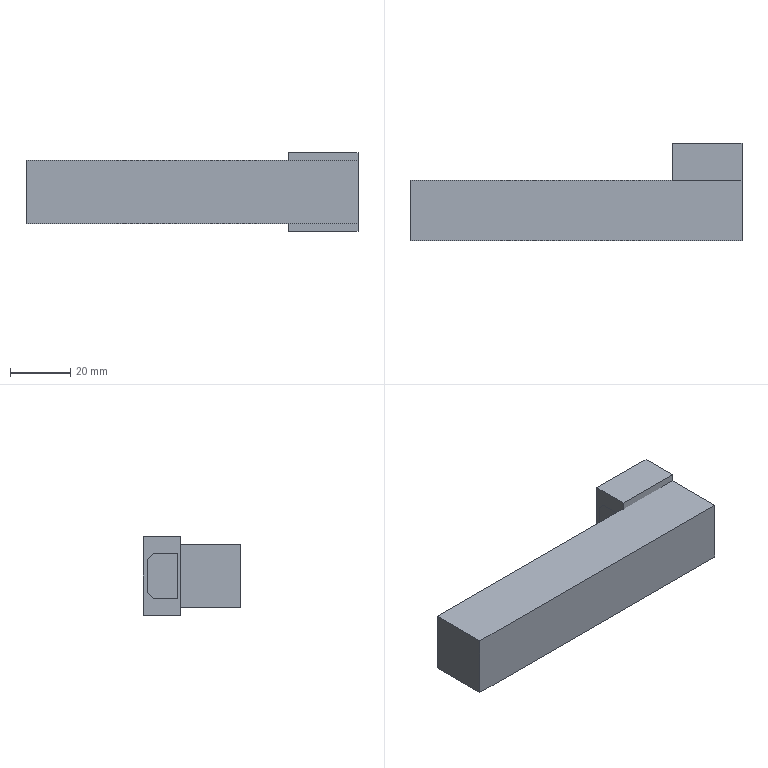NC program | NX | posted with a generic post | part box 110 x 32.2 x 26 mm
Lines 4082 to 5595 of 5595, first 1420 of 1508 lines:
(PLANAR_MILL_10 , TOOL : D4C)
N8030 T03 M6
N8032 G54
N8034 G17 G0 G90 X8.566 Y-0.32 S3000 M3
N8036 G43 Z20. H3
N8038 Z-1.8
N8040 G94 G1 X8.819 Y-0.529 Z-1.806 F1000.
N8042 X9.181 Z-1.812
N8044 X9.484 Y-0.279 Z-1.819
N8046 X9.548 Y0.108 Z-1.826
N8048 X9.367 Y0.421 Z-1.832
N8050 X9.181 Y0.529 Z-1.836
N8052 X8.819 Z-1.842
N8054 X8.633 Y0.421 Z-1.846
N8056 X8.452 Y0.108 Z-1.852
N8058 X8.516 Y-0.279 Z-1.859
N8060 X8.819 Y-0.529 Z-1.866
N8062 X9.181 Z-1.872
N8064 X9.484 Y-0.279 Z-1.879
N8066 X9.548 Y0.108 Z-1.886
N8068 X9.367 Y0.421 Z-1.892
N8070 X9.181 Y0.529 Z-1.896
N8072 X8.819 Z-1.902
N8074 X8.633 Y0.421 Z-1.906
N8076 X8.452 Y0.108 Z-1.912
N8078 X8.516 Y-0.279 Z-1.919
N8080 X8.819 Y-0.529 Z-1.926
N8082 X9.181 Z-1.932
N8084 X9.484 Y-0.279 Z-1.939
N8086 X9.548 Y0.108 Z-1.946
N8088 X9.367 Y0.421 Z-1.952
N8090 X9.181 Y0.529 Z-1.956
N8092 X8.819 Z-1.962
N8094 X8.633 Y0.421 Z-1.966
N8096 X8.452 Y0.108 Z-1.972
N8098 X8.516 Y-0.279 Z-1.979
N8100 X8.819 Y-0.529 Z-1.986
N8102 X9.181 Z-1.992
N8104 X9.484 Y-0.279 Z-1.999
N8106 X9.548 Y0.108 Z-2.006
N8108 X9.367 Y0.421 Z-2.012
N8110 X9.181 Y0.529 Z-2.016
N8112 X8.819 Z-2.023
N8114 X8.633 Y0.421 Z-2.026
N8116 X8.452 Y0.108 Z-2.033
N8118 X8.516 Y-0.279 Z-2.039
N8120 X8.819 Y-0.529 Z-2.046
N8122 X9.181 Z-2.053
N8124 X9.484 Y-0.279 Z-2.059
N8126 X9.548 Y0.108 Z-2.066
N8128 X9.367 Y0.421 Z-2.073
N8130 X9.181 Y0.529 Z-2.076
N8132 X8.819 Z-2.083
N8134 X8.633 Y0.421 Z-2.086
N8136 X8.452 Y0.108 Z-2.093
N8138 X8.516 Y-0.279 Z-2.1
N8140 X8.819 Y-0.529 Z-2.106
N8142 X9.181 Z-2.113
N8144 X9.484 Y-0.279 Z-2.12
N8146 X9.548 Y0.108 Z-2.126
N8148 X9.367 Y0.421 Z-2.133
N8150 X9.181 Y0.529 Z-2.137
N8152 X8.819 Z-2.143
N8154 X8.633 Y0.421 Z-2.147
N8156 X8.452 Y0.108 Z-2.153
N8158 X8.516 Y-0.279 Z-2.16
N8160 X8.819 Y-0.529 Z-2.167
N8162 X9.181 Z-2.173
N8164 X9.484 Y-0.279 Z-2.18
N8166 X9.548 Y0.108 Z-2.187
N8168 X9.367 Y0.421 Z-2.193
N8170 X9.181 Y0.529 Z-2.197
N8172 X8.819 Z-2.203
N8174 X8.633 Y0.421 Z-2.207
N8176 X8.452 Y0.108 Z-2.213
N8178 X8.516 Y-0.279 Z-2.22
N8180 X8.819 Y-0.529 Z-2.227
N8182 X9.181 Z-2.233
N8184 X9.484 Y-0.279 Z-2.24
N8186 X9.548 Y0.108 Z-2.247
N8188 X9.367 Y0.421 Z-2.253
N8190 X9.181 Y0.529 Z-2.257
N8192 X8.819 Z-2.263
N8194 X8.633 Y0.421 Z-2.267
N8196 X8.452 Y0.108 Z-2.273
N8198 X8.516 Y-0.279 Z-2.28
N8200 X8.819 Y-0.529 Z-2.287
N8202 X9.181 Z-2.293
N8204 X9.484 Y-0.279 Z-2.3
N8206 X9.548 Y0.108 Z-2.307
N8208 X9.367 Y0.421 Z-2.313
N8210 X9.181 Y0.529 Z-2.317
N8212 X8.819 Z-2.323
N8214 X8.633 Y0.421 Z-2.327
N8216 X8.452 Y0.108 Z-2.333
N8218 X8.516 Y-0.279 Z-2.34
N8220 X8.819 Y-0.529 Z-2.347
N8222 X9.181 Z-2.353
N8224 X9.484 Y-0.279 Z-2.36
N8226 X9.548 Y0.108 Z-2.367
N8228 X9.367 Y0.421 Z-2.373
N8230 X9.181 Y0.529 Z-2.377
N8232 X8.819 Z-2.383
N8234 X8.633 Y0.421 Z-2.387
N8236 X8.452 Y0.108 Z-2.393
N8238 X8.516 Y-0.279 Z-2.4
N8240 X8.819 Y-0.529 Z-2.407
N8242 X9.181 Z-2.413
N8244 X9.484 Y-0.279 Z-2.42
N8246 X9.548 Y0.108 Z-2.427
N8248 X9.367 Y0.421 Z-2.434
N8250 X9.181 Y0.529 Z-2.437
N8252 X8.819 Z-2.444
N8254 X8.633 Y0.421 Z-2.447
N8256 X8.452 Y0.108 Z-2.454
N8258 X8.516 Y-0.279 Z-2.46
N8260 X8.819 Y-0.529 Z-2.467
N8262 X9.181 Z-2.474
N8264 X9.484 Y-0.279 Z-2.48
N8266 X9.548 Y0.108 Z-2.487
N8268 X9.367 Y0.421 Z-2.494
N8270 X9.181 Y0.529 Z-2.497
N8272 X8.819 Z-2.504
N8274 X8.633 Y0.421 Z-2.507
N8276 X8.452 Y0.108 Z-2.514
N8278 X8.516 Y-0.279 Z-2.521
N8280 X8.819 Y-0.529 Z-2.527
N8282 X9.181 Z-2.534
N8284 X9.484 Y-0.279 Z-2.541
N8286 X9.548 Y0.108 Z-2.547
N8288 X9.367 Y0.421 Z-2.554
N8290 X9.181 Y0.529 Z-2.558
N8292 X8.819 Z-2.564
N8294 X8.633 Y0.421 Z-2.568
N8296 X8.452 Y0.108 Z-2.574
N8298 X8.516 Y-0.279 Z-2.581
N8300 X8.819 Y-0.529 Z-2.588
N8302 X9.181 Z-2.594
N8304 X9.484 Y-0.279 Z-2.601
N8306 X9.548 Y0.108 Z-2.608
N8308 X9.367 Y0.421 Z-2.614
N8310 X9.181 Y0.529 Z-2.618
N8312 X8.819 Z-2.624
N8314 X8.633 Y0.421 Z-2.628
N8316 X8.452 Y0.108 Z-2.634
N8318 X8.516 Y-0.279 Z-2.641
N8320 X8.819 Y-0.529 Z-2.648
N8322 X9.181 Z-2.654
N8324 X9.484 Y-0.279 Z-2.661
N8326 X9.548 Y0.108 Z-2.668
N8328 X9.367 Y0.421 Z-2.674
N8330 X9.181 Y0.529 Z-2.678
N8332 X8.819 Z-2.684
N8334 X8.633 Y0.421 Z-2.688
N8336 X8.452 Y0.108 Z-2.694
N8338 X8.516 Y-0.279 Z-2.701
N8340 X8.819 Y-0.529 Z-2.708
N8342 X9.181 Z-2.714
N8344 X9.484 Y-0.279 Z-2.721
N8346 X9.548 Y0.108 Z-2.728
N8348 X9.367 Y0.421 Z-2.734
N8350 X9.181 Y0.529 Z-2.738
N8352 X8.819 Z-2.744
N8354 X8.633 Y0.421 Z-2.748
N8356 X8.452 Y0.108 Z-2.754
N8358 X8.516 Y-0.279 Z-2.761
N8360 X8.819 Y-0.529 Z-2.768
N8362 X9.181 Z-2.774
N8364 X9.484 Y-0.279 Z-2.781
N8366 X9.548 Y0.108 Z-2.788
N8368 X9.367 Y0.421 Z-2.794
N8370 X9.181 Y0.529 Z-2.798
N8372 X8.819 Z-2.804
N8374 X8.633 Y0.421 Z-2.808
N8376 X8.452 Y0.108 Z-2.815
N8378 X8.516 Y-0.279 Z-2.821
N8380 X8.819 Y-0.529 Z-2.828
N8382 X9.181 Z-2.835
N8384 X9.484 Y-0.279 Z-2.841
N8386 X9.548 Y0.108 Z-2.848
N8388 X9.367 Y0.421 Z-2.855
N8390 X9.181 Y0.529 Z-2.858
N8392 X8.819 Z-2.865
N8394 X8.633 Y0.421 Z-2.868
N8396 X8.452 Y0.108 Z-2.875
N8398 X8.516 Y-0.279 Z-2.882
N8400 X8.819 Y-0.529 Z-2.888
N8402 X9.181 Z-2.895
N8404 X9.484 Y-0.279 Z-2.902
N8406 X9.548 Y0.108 Z-2.908
N8408 X9.367 Y0.421 Z-2.915
N8410 X9.181 Y0.529 Z-2.918
N8412 X8.819 Z-2.925
N8414 X8.633 Y0.421 Z-2.929
N8416 X8.452 Y0.108 Z-2.935
N8418 X8.516 Y-0.279 Z-2.942
N8420 X8.819 Y-0.529 Z-2.949
N8422 X9.181 Z-2.955
N8424 X9.484 Y-0.279 Z-2.962
N8426 X9.548 Y0.108 Z-2.969
N8428 X9.367 Y0.421 Z-2.975
N8430 X9.181 Y0.529 Z-2.979
N8432 X8.819 Z-2.985
N8434 X8.633 Y0.421 Z-2.989
N8436 X8.452 Y0.108 Z-2.995
N8438 X8.516 Y-0.279 Z-3.002
N8440 X8.819 Y-0.529 Z-3.009
N8442 X9.181 Z-3.015
N8444 X9.484 Y-0.279 Z-3.022
N8446 X9.548 Y0.108 Z-3.029
N8448 X9.367 Y0.421 Z-3.035
N8450 X9.181 Y0.529 Z-3.039
N8452 X8.819 Z-3.045
N8454 X8.633 Y0.421 Z-3.049
N8456 X8.452 Y0.108 Z-3.055
N8458 X8.516 Y-0.279 Z-3.062
N8460 X8.819 Y-0.529 Z-3.069
N8462 X9.181 Z-3.075
N8464 X9.484 Y-0.279 Z-3.082
N8466 X9.548 Y0.108 Z-3.089
N8468 X9.367 Y0.421 Z-3.095
N8470 X9.181 Y0.529 Z-3.099
N8472 X8.819 Z-3.105
N8474 X8.633 Y0.421 Z-3.109
N8476 X8.452 Y0.108 Z-3.115
N8478 X8.516 Y-0.279 Z-3.122
N8480 X8.819 Y-0.529 Z-3.129
N8482 X9.181 Z-3.135
N8484 X9.484 Y-0.279 Z-3.142
N8486 X9.548 Y0.108 Z-3.149
N8488 X9.367 Y0.421 Z-3.155
N8490 X9.181 Y0.529 Z-3.159
N8492 X8.819 Z-3.165
N8494 X8.633 Y0.421 Z-3.169
N8496 X8.452 Y0.108 Z-3.175
N8498 X8.516 Y-0.279 Z-3.182
N8500 X8.819 Y-0.529 Z-3.189
N8502 X9.181 Z-3.195
N8504 X9.484 Y-0.279 Z-3.202
N8506 X9.548 Y0.108 Z-3.209
N8508 X9.367 Y0.421 Z-3.215
N8510 X9.181 Y0.529 Z-3.219
N8512 X8.819 Z-3.225
N8514 X8.633 Y0.421 Z-3.229
N8516 X8.452 Y0.108 Z-3.236
N8518 X8.516 Y-0.279 Z-3.242
N8520 X8.819 Y-0.529 Z-3.249
N8522 X9.181 Z-3.256
N8524 X9.484 Y-0.279 Z-3.262
N8526 X9.548 Y0.108 Z-3.269
N8528 X9.367 Y0.421 Z-3.276
N8530 X9.181 Y0.529 Z-3.279
N8532 X8.819 Z-3.286
N8534 X8.633 Y0.421 Z-3.289
N8536 X8.452 Y0.108 Z-3.296
N8538 X8.516 Y-0.279 Z-3.303
N8540 X8.819 Y-0.529 Z-3.309
N8542 X9.181 Z-3.316
N8544 X9.484 Y-0.279 Z-3.323
N8546 X9.548 Y0.108 Z-3.329
N8548 X9.367 Y0.421 Z-3.336
N8550 X9.181 Y0.529 Z-3.339
N8552 X8.819 Z-3.346
N8554 X8.633 Y0.421 Z-3.35
N8556 X8.452 Y0.108 Z-3.356
N8558 X8.516 Y-0.279 Z-3.363
N8560 X8.819 Y-0.529 Z-3.37
N8562 X9.181 Z-3.376
N8564 X9.484 Y-0.279 Z-3.383
N8566 X9.548 Y0.108 Z-3.39
N8568 X9.367 Y0.421 Z-3.396
N8570 X9.181 Y0.529 Z-3.4
N8572 X8.819 Z-3.406
N8574 X8.633 Y0.421 Z-3.41
N8576 X8.452 Y0.108 Z-3.416
N8578 X8.516 Y-0.279 Z-3.423
N8580 X8.819 Y-0.529 Z-3.43
N8582 X9.181 Z-3.436
N8584 X9.484 Y-0.279 Z-3.443
N8586 X9.548 Y0.108 Z-3.45
N8588 X9.367 Y0.421 Z-3.456
N8590 X9.181 Y0.529 Z-3.46
N8592 X8.819 Z-3.466
N8594 X8.633 Y0.421 Z-3.47
N8596 X8.452 Y0.108 Z-3.476
N8598 X8.516 Y-0.279 Z-3.483
N8600 X8.819 Y-0.529 Z-3.49
N8602 X9.181 Z-3.496
N8604 X9.484 Y-0.279 Z-3.503
N8606 X9.548 Y0.108 Z-3.51
N8608 X9.367 Y0.421 Z-3.516
N8610 X9.181 Y0.529 Z-3.52
N8612 X8.819 Z-3.526
N8614 X8.633 Y0.421 Z-3.53
N8616 X8.452 Y0.108 Z-3.536
N8618 X8.516 Y-0.279 Z-3.543
N8620 X8.819 Y-0.529 Z-3.55
N8622 X9.181 Z-3.556
N8624 X9.484 Y-0.279 Z-3.563
N8626 X9.548 Y0.108 Z-3.57
N8628 X9.367 Y0.421 Z-3.576
N8630 X9.181 Y0.529 Z-3.58
N8632 X8.819 Z-3.586
N8634 X8.633 Y0.421 Z-3.59
N8636 X8.452 Y0.108 Z-3.596
N8638 X8.516 Y-0.279 Z-3.603
N8640 X8.819 Y-0.529 Z-3.61
N8642 X9.181 Z-3.616
N8644 X9.484 Y-0.279 Z-3.623
N8646 X9.548 Y0.108 Z-3.63
N8648 X9.367 Y0.421 Z-3.636
N8650 X9.181 Y0.529 Z-3.64
N8652 X8.819 Z-3.646
N8654 X8.633 Y0.421 Z-3.65
N8656 X8.452 Y0.108 Z-3.657
N8658 X8.516 Y-0.279 Z-3.663
N8660 X8.819 Y-0.529 Z-3.67
N8662 X9.181 Z-3.677
N8664 X9.484 Y-0.279 Z-3.683
N8666 X9.548 Y0.108 Z-3.69
N8668 X9.367 Y0.421 Z-3.697
N8670 X9.181 Y0.529 Z-3.7
N8672 X8.819 Z-3.707
N8674 X8.633 Y0.421 Z-3.71
N8676 X8.452 Y0.108 Z-3.717
N8678 X8.516 Y-0.279 Z-3.724
N8680 X8.819 Y-0.529 Z-3.73
N8682 X9.181 Z-3.737
N8684 X9.484 Y-0.279 Z-3.744
N8686 X9.548 Y0.108 Z-3.75
N8688 X9.367 Y0.421 Z-3.757
N8690 X9.181 Y0.529 Z-3.76
N8692 X8.819 Z-3.767
N8694 X8.633 Y0.421 Z-3.771
N8696 X8.452 Y0.108 Z-3.777
N8698 X8.516 Y-0.279 Z-3.784
N8700 X8.819 Y-0.529 Z-3.791
N8702 X9.181 Z-3.797
N8704 X9.484 Y-0.279 Z-3.804
N8706 X9.548 Y0.108 Z-3.811
N8708 X9.367 Y0.421 Z-3.817
N8710 X9.181 Y0.529 Z-3.821
N8712 X8.819 Z-3.827
N8714 X8.633 Y0.421 Z-3.831
N8716 X8.452 Y0.108 Z-3.837
N8718 X8.516 Y-0.279 Z-3.844
N8720 X8.819 Y-0.529 Z-3.851
N8722 X9.181 Z-3.857
N8724 X9.484 Y-0.279 Z-3.864
N8726 X9.548 Y0.108 Z-3.871
N8728 X9.367 Y0.421 Z-3.877
N8730 X9.181 Y0.529 Z-3.881
N8732 X8.819 Z-3.887
N8734 X8.633 Y0.421 Z-3.891
N8736 X8.452 Y0.108 Z-3.897
N8738 X8.516 Y-0.279 Z-3.904
N8740 X8.819 Y-0.529 Z-3.911
N8742 X9.181 Z-3.917
N8744 X9.484 Y-0.279 Z-3.924
N8746 X9.548 Y0.108 Z-3.931
N8748 X9.367 Y0.421 Z-3.937
N8750 X9.181 Y0.529 Z-3.941
N8752 X8.819 Z-3.947
N8754 X8.633 Y0.421 Z-3.951
N8756 X8.452 Y0.108 Z-3.957
N8758 X8.516 Y-0.279 Z-3.964
N8760 X8.819 Y-0.529 Z-3.971
N8762 X9.181 Z-3.977
N8764 X9.484 Y-0.279 Z-3.984
N8766 X9.548 Y0.108 Z-3.991
N8768 X9.367 Y0.421 Z-3.997
N8770 X9.181 Y0.529 Z-4.001
N8772 X8.819 Z-4.007
N8774 X8.633 Y0.421 Z-4.011
N8776 X8.452 Y0.108 Z-4.017
N8778 X8.516 Y-0.279 Z-4.024
N8780 X8.819 Y-0.529 Z-4.031
N8782 X9.181 Z-4.037
N8784 X9.484 Y-0.279 Z-4.044
N8786 X9.548 Y0.108 Z-4.051
N8788 X9.367 Y0.421 Z-4.057
N8790 X9.181 Y0.529 Z-4.061
N8792 X8.819 Z-4.068
N8794 X8.633 Y0.421 Z-4.071
N8796 X8.452 Y0.108 Z-4.078
N8798 X8.516 Y-0.279 Z-4.084
N8800 X8.819 Y-0.529 Z-4.091
N8802 X9.181 Z-4.098
N8804 X9.484 Y-0.279 Z-4.104
N8806 X9.548 Y0.108 Z-4.111
N8808 X9.367 Y0.421 Z-4.118
N8810 X9.181 Y0.529 Z-4.121
N8812 X8.819 Z-4.128
N8814 X8.633 Y0.421 Z-4.131
N8816 X8.452 Y0.108 Z-4.138
N8818 X8.516 Y-0.279 Z-4.145
N8820 X8.819 Y-0.529 Z-4.151
N8822 X9.181 Z-4.158
N8824 X9.484 Y-0.279 Z-4.165
N8826 X9.548 Y0.108 Z-4.171
N8828 X9.367 Y0.421 Z-4.178
N8830 X9.181 Y0.529 Z-4.182
N8832 X8.819 Z-4.188
N8834 X8.633 Y0.421 Z-4.192
N8836 X8.452 Y0.108 Z-4.198
N8838 X8.516 Y-0.279 Z-4.205
N8840 X8.819 Y-0.529 Z-4.212
N8842 X9.181 Z-4.218
N8844 X9.484 Y-0.279 Z-4.225
N8846 X9.548 Y0.108 Z-4.232
N8848 X9.367 Y0.421 Z-4.238
N8850 X9.181 Y0.529 Z-4.242
N8852 X8.819 Z-4.248
N8854 X8.633 Y0.421 Z-4.252
N8856 X8.452 Y0.108 Z-4.258
N8858 X8.516 Y-0.279 Z-4.265
N8860 X8.819 Y-0.529 Z-4.272
N8862 X9.181 Z-4.278
N8864 X9.484 Y-0.279 Z-4.285
N8866 X9.548 Y0.108 Z-4.292
N8868 X9.367 Y0.421 Z-4.298
N8870 X9.181 Y0.529 Z-4.302
N8872 X8.819 Z-4.308
N8874 X8.633 Y0.421 Z-4.312
N8876 X8.452 Y0.108 Z-4.318
N8878 X8.516 Y-0.279 Z-4.325
N8880 X8.819 Y-0.529 Z-4.332
N8882 X9.181 Z-4.338
N8884 X9.484 Y-0.279 Z-4.345
N8886 X9.548 Y0.108 Z-4.352
N8888 X9.367 Y0.421 Z-4.358
N8890 X9.181 Y0.529 Z-4.362
N8892 X8.819 Z-4.368
N8894 X8.633 Y0.421 Z-4.372
N8896 X8.452 Y0.108 Z-4.378
N8898 X8.516 Y-0.279 Z-4.385
N8900 X8.819 Y-0.529 Z-4.392
N8902 X9.181 Z-4.398
N8904 X9.484 Y-0.279 Z-4.405
N8906 X9.548 Y0.108 Z-4.412
N8908 X9.367 Y0.421 Z-4.418
N8910 X9.181 Y0.529 Z-4.422
N8912 X8.819 Z-4.428
N8914 X8.633 Y0.421 Z-4.432
N8916 X8.452 Y0.108 Z-4.438
N8918 X8.516 Y-0.279 Z-4.445
N8920 X8.819 Y-0.529 Z-4.452
N8922 X9.181 Z-4.458
N8924 X9.484 Y-0.279 Z-4.465
N8926 X9.548 Y0.108 Z-4.472
N8928 X9.367 Y0.421 Z-4.478
N8930 X9.181 Y0.529 Z-4.482
N8932 X8.819 Z-4.489
N8934 X8.633 Y0.421 Z-4.492
N8936 X8.452 Y0.108 Z-4.499
N8938 X8.516 Y-0.279 Z-4.505
N8940 X8.819 Y-0.529 Z-4.512
N8942 X9.181 Z-4.519
N8944 X9.484 Y-0.279 Z-4.525
N8946 X9.548 Y0.108 Z-4.532
N8948 X9.367 Y0.421 Z-4.539
N8950 X9.181 Y0.529 Z-4.542
N8952 X8.819 Z-4.549
N8954 X8.633 Y0.421 Z-4.552
N8956 X8.452 Y0.108 Z-4.559
N8958 X8.516 Y-0.279 Z-4.566
N8960 X8.819 Y-0.529 Z-4.572
N8962 X9.181 Z-4.579
N8964 X9.484 Y-0.279 Z-4.586
N8966 X9.548 Y0.108 Z-4.592
N8968 X9.367 Y0.421 Z-4.599
N8970 X9.181 Y0.529 Z-4.603
N8972 X8.819 Z-4.609
N8974 X8.633 Y0.421 Z-4.613
N8976 X8.452 Y0.108 Z-4.619
N8978 X8.516 Y-0.279 Z-4.626
N8980 X8.819 Y-0.529 Z-4.633
N8982 X9.181 Z-4.639
N8984 X9.484 Y-0.279 Z-4.646
N8986 X9.548 Y0.108 Z-4.653
N8988 X9.367 Y0.421 Z-4.659
N8990 X9.181 Y0.529 Z-4.663
N8992 X8.819 Z-4.669
N8994 X8.633 Y0.421 Z-4.673
N8996 X8.452 Y0.108 Z-4.679
N8998 X8.516 Y-0.279 Z-4.686
N9000 X8.819 Y-0.529 Z-4.693
N9002 X9.181 Z-4.699
N9004 X9.484 Y-0.279 Z-4.706
N9006 X9.548 Y0.108 Z-4.713
N9008 X9.367 Y0.421 Z-4.719
N9010 X9.181 Y0.529 Z-4.723
N9012 X8.819 Z-4.729
N9014 X8.633 Y0.421 Z-4.733
N9016 X8.452 Y0.108 Z-4.739
N9018 X8.516 Y-0.279 Z-4.746
N9020 X8.819 Y-0.529 Z-4.753
N9022 X9.181 Z-4.759
N9024 X9.484 Y-0.279 Z-4.766
N9026 X9.548 Y0.108 Z-4.773
N9028 X9.367 Y0.421 Z-4.779
N9030 X9.181 Y0.529 Z-4.783
N9032 X8.819 Z-4.789
N9034 X8.633 Y0.421 Z-4.793
N9036 X8.452 Y0.108 Z-4.799
N9038 X8.516 Y-0.279 Z-4.806
N9040 X8.819 Y-0.529 Z-4.813
N9042 X9.181 Z-4.819
N9044 X9.484 Y-0.279 Z-4.826
N9046 X9.548 Y0.108 Z-4.833
N9048 X9.367 Y0.421 Z-4.839
N9050 X9.181 Y0.529 Z-4.843
N9052 X8.819 Z-4.849
N9054 X8.633 Y0.421 Z-4.853
N9056 X8.452 Y0.108 Z-4.859
N9058 X8.516 Y-0.279 Z-4.866
N9060 X8.819 Y-0.529 Z-4.873
N9062 X9.181 Z-4.879
N9064 X9.484 Y-0.279 Z-4.886
N9066 X9.548 Y0.108 Z-4.893
N9068 X9.367 Y0.421 Z-4.899
N9070 X9.181 Y0.529 Z-4.903
N9072 X8.819 Z-4.91
N9074 X8.633 Y0.421 Z-4.913
N9076 X8.452 Y0.108 Z-4.92
N9078 X8.516 Y-0.279 Z-4.926
N9080 X8.819 Y-0.529 Z-4.933
N9082 X9.181 Z-4.94
N9084 X9.484 Y-0.279 Z-4.946
N9086 X9.548 Y0.108 Z-4.953
N9088 X9.367 Y0.421 Z-4.96
N9090 X9.181 Y0.529 Z-4.963
N9092 X8.819 Z-4.97
N9094 X8.633 Y0.421 Z-4.973
N9096 X8.452 Y0.108 Z-4.98
N9098 X8.516 Y-0.279 Z-4.987
N9100 X8.819 Y-0.529 Z-4.993
N9102 X9.181 Z-5.
N9104 X9.484 Y-0.279 Z-5.007
N9106 X9.548 Y0.108 Z-5.013
N9108 X9.367 Y0.421 Z-5.02
N9110 X9.181 Y0.529 Z-5.024
N9112 X8.819 Z-5.03
N9114 X8.633 Y0.421 Z-5.034
N9116 X8.452 Y0.108 Z-5.04
N9118 X8.516 Y-0.279 Z-5.047
N9120 X8.819 Y-0.529 Z-5.054
N9122 X9.181 Z-5.06
N9124 X9.484 Y-0.279 Z-5.067
N9126 X9.548 Y0.108 Z-5.074
N9128 X9.367 Y0.421 Z-5.08
N9130 X9.181 Y0.529 Z-5.084
N9132 X8.819 Z-5.09
N9134 X8.633 Y0.421 Z-5.094
N9136 X8.452 Y0.108 Z-5.1
N9138 X8.516 Y-0.279 Z-5.107
N9140 X8.819 Y-0.529 Z-5.114
N9142 X9.181 Z-5.12
N9144 X9.484 Y-0.279 Z-5.127
N9146 X9.548 Y0.108 Z-5.134
N9148 X9.367 Y0.421 Z-5.14
N9150 X9.181 Y0.529 Z-5.144
N9152 X8.819 Z-5.15
N9154 X8.633 Y0.421 Z-5.154
N9156 X8.452 Y0.108 Z-5.16
N9158 X8.516 Y-0.279 Z-5.167
N9160 X8.819 Y-0.529 Z-5.174
N9162 X9.181 Z-5.18
N9164 X9.484 Y-0.279 Z-5.187
N9166 X9.548 Y0.108 Z-5.194
N9168 X9.367 Y0.421 Z-5.2
N9170 X9.181 Y0.529 Z-5.204
N9172 X8.819 Z-5.21
N9174 X8.633 Y0.421 Z-5.214
N9176 X8.452 Y0.108 Z-5.22
N9178 X8.516 Y-0.279 Z-5.227
N9180 X8.819 Y-0.529 Z-5.234
N9182 X9.181 Z-5.24
N9184 X9.484 Y-0.279 Z-5.247
N9186 X9.548 Y0.108 Z-5.254
N9188 X9.367 Y0.421 Z-5.26
N9190 X9.181 Y0.529 Z-5.264
N9192 X8.819 Z-5.27
N9194 X8.633 Y0.421 Z-5.274
N9196 X8.452 Y0.108 Z-5.281
N9198 X8.516 Y-0.279 Z-5.287
N9200 X8.819 Y-0.529 Z-5.294
N9202 X9.181 Z-5.301
N9204 X9.484 Y-0.279 Z-5.307
N9206 X9.548 Y0.108 Z-5.314
N9208 X9.367 Y0.421 Z-5.321
N9210 X9.181 Y0.529 Z-5.324
N9212 X8.819 Z-5.331
N9214 X8.633 Y0.421 Z-5.334
N9216 X8.452 Y0.108 Z-5.341
N9218 X8.516 Y-0.279 Z-5.348
N9220 X8.819 Y-0.529 Z-5.354
N9222 X9.181 Z-5.361
N9224 X9.484 Y-0.279 Z-5.368
N9226 X9.548 Y0.108 Z-5.374
N9228 X9.367 Y0.421 Z-5.381
N9230 X9.181 Y0.529 Z-5.384
N9232 X8.819 Z-5.391
N9234 X8.633 Y0.421 Z-5.394
N9236 X8.452 Y0.108 Z-5.401
N9238 X8.516 Y-0.279 Z-5.408
N9240 X8.819 Y-0.529 Z-5.415
N9242 X9.181 Z-5.421
N9244 X9.484 Y-0.279 Z-5.428
N9246 X9.548 Y0.108 Z-5.435
N9248 X9.367 Y0.421 Z-5.441
N9250 X9.181 Y0.529 Z-5.445
N9252 X8.819 Z-5.451
N9254 X8.633 Y0.421 Z-5.455
N9256 X8.452 Y0.108 Z-5.461
N9258 X8.516 Y-0.279 Z-5.468
N9260 X8.819 Y-0.529 Z-5.475
N9262 X9.181 Z-5.481
N9264 X9.484 Y-0.279 Z-5.488
N9266 X9.548 Y0.108 Z-5.495
N9268 X9.367 Y0.421 Z-5.501
N9270 X9.181 Y0.529 Z-5.505
N9272 X8.819 Z-5.511
N9274 X8.633 Y0.421 Z-5.515
N9276 X8.452 Y0.108 Z-5.521
N9278 X8.516 Y-0.279 Z-5.528
N9280 X8.819 Y-0.529 Z-5.535
N9282 X9.181 Z-5.541
N9284 X9.484 Y-0.279 Z-5.548
N9286 X9.548 Y0.108 Z-5.555
N9288 X9.367 Y0.421 Z-5.561
N9290 X9.181 Y0.529 Z-5.565
N9292 X8.819 Z-5.571
N9294 X8.633 Y0.421 Z-5.575
N9296 X8.452 Y0.108 Z-5.581
N9298 X8.516 Y-0.279 Z-5.588
N9300 X8.819 Y-0.529 Z-5.595
N9302 X9.181 Z-5.601
N9304 X9.484 Y-0.279 Z-5.608
N9306 X9.548 Y0.108 Z-5.615
N9308 X9.367 Y0.421 Z-5.621
N9310 X9.181 Y0.529 Z-5.625
N9312 X8.819 Z-5.631
N9314 X8.633 Y0.421 Z-5.635
N9316 X8.452 Y0.108 Z-5.641
N9318 X8.516 Y-0.279 Z-5.648
N9320 X8.819 Y-0.529 Z-5.655
N9322 X9.181 Z-5.661
N9324 X9.484 Y-0.279 Z-5.668
N9326 X9.548 Y0.108 Z-5.675
N9328 X9.367 Y0.421 Z-5.681
N9330 X9.181 Y0.529 Z-5.685
N9332 X8.819 Z-5.691
N9334 X8.633 Y0.421 Z-5.695
N9336 X8.452 Y0.108 Z-5.702
N9338 X8.516 Y-0.279 Z-5.708
N9340 X8.819 Y-0.529 Z-5.715
N9342 X9.181 Z-5.722
N9344 X9.484 Y-0.279 Z-5.728
N9346 X9.548 Y0.108 Z-5.735
N9348 X9.367 Y0.421 Z-5.742
N9350 X9.181 Y0.529 Z-5.745
N9352 X8.819 Z-5.752
N9354 X8.633 Y0.421 Z-5.755
N9356 X8.452 Y0.108 Z-5.762
N9358 X8.516 Y-0.279 Z-5.769
N9360 X8.819 Y-0.529 Z-5.775
N9362 X9.181 Z-5.782
N9364 X9.484 Y-0.279 Z-5.789
N9366 X9.548 Y0.108 Z-5.795
N9368 X9.367 Y0.421 Z-5.802
N9370 X9.181 Y0.529 Z-5.805
N9372 X8.819 Z-5.812
N9374 X8.633 Y0.421 Z-5.816
N9376 X8.452 Y0.108 Z-5.822
N9378 X8.516 Y-0.279 Z-5.829
N9380 X8.819 Y-0.529 Z-5.836
N9382 X9.181 Z-5.842
N9384 X9.484 Y-0.279 Z-5.849
N9386 X9.548 Y0.108 Z-5.856
N9388 X9.367 Y0.421 Z-5.862
N9390 X9.181 Y0.529 Z-5.866
N9392 X8.819 Z-5.872
N9394 X8.633 Y0.421 Z-5.876
N9396 X8.452 Y0.108 Z-5.882
N9398 X8.516 Y-0.279 Z-5.889
N9400 X8.819 Y-0.529 Z-5.896
N9402 X9.181 Z-5.902
N9404 X9.484 Y-0.279 Z-5.909
N9406 X9.548 Y0.108 Z-5.916
N9408 X9.367 Y0.421 Z-5.922
N9410 X9.181 Y0.529 Z-5.926
N9412 X8.819 Z-5.932
N9414 X8.633 Y0.421 Z-5.936
N9416 X8.452 Y0.108 Z-5.942
N9418 X8.516 Y-0.279 Z-5.949
N9420 X8.819 Y-0.529 Z-5.956
N9422 X9.181 Z-5.962
N9424 X9.484 Y-0.279 Z-5.969
N9426 X9.548 Y0.108 Z-5.976
N9428 X9.367 Y0.421 Z-5.982
N9430 X9.181 Y0.529 Z-5.986
N9432 X8.819 Z-5.992
N9434 X8.633 Y0.421 Z-5.996
N9436 X8.452 Y0.108 Z-6.002
N9438 X8.516 Y-0.279 Z-6.009
N9440 X8.819 Y-0.529 Z-6.016
N9442 X9.181 Z-6.022
N9444 X9.484 Y-0.279 Z-6.029
N9446 X9.548 Y0.108 Z-6.036
N9448 X9.367 Y0.421 Z-6.042
N9450 X9.181 Y0.529 Z-6.046
N9452 X8.819 Z-6.052
N9454 X8.633 Y0.421 Z-6.056
N9456 X8.452 Y0.108 Z-6.062
N9458 X8.516 Y-0.279 Z-6.069
N9460 X8.819 Y-0.529 Z-6.076
N9462 X9.181 Z-6.082
N9464 X9.484 Y-0.279 Z-6.089
N9466 X9.548 Y0.108 Z-6.096
N9468 X9.367 Y0.421 Z-6.102
N9470 X9.181 Y0.529 Z-6.106
N9472 X8.819 Z-6.112
N9474 X8.633 Y0.421 Z-6.116
N9476 X8.452 Y0.108 Z-6.123
N9478 X8.516 Y-0.279 Z-6.129
N9480 X8.819 Y-0.529 Z-6.136
N9482 X9.181 Z-6.143
N9484 X9.484 Y-0.279 Z-6.149
N9486 X9.548 Y0.108 Z-6.156
N9488 X9.367 Y0.421 Z-6.163
N9490 X9.181 Y0.529 Z-6.166
N9492 X8.819 Z-6.173
N9494 X8.633 Y0.421 Z-6.176
N9496 X8.452 Y0.108 Z-6.183
N9498 X8.516 Y-0.279 Z-6.19
N9500 X8.819 Y-0.529 Z-6.196
N9502 X9.181 Z-6.203
N9504 X9.484 Y-0.279 Z-6.21
N9506 X9.548 Y0.108 Z-6.216
N9508 X9.367 Y0.421 Z-6.223
N9510 X9.181 Y0.529 Z-6.226
N9512 X8.819 Z-6.233
N9514 X8.633 Y0.421 Z-6.237
N9516 X8.452 Y0.108 Z-6.243
N9518 X8.516 Y-0.279 Z-6.25
N9520 X8.819 Y-0.529 Z-6.257
N9522 X9.181 Z-6.263
N9524 X9.484 Y-0.279 Z-6.27
N9526 X9.548 Y0.108 Z-6.277
N9528 X9.367 Y0.421 Z-6.283
N9530 X9.181 Y0.529 Z-6.287
N9532 X8.819 Z-6.293
N9534 X8.633 Y0.421 Z-6.297
N9536 X8.452 Y0.108 Z-6.303
N9538 X8.516 Y-0.279 Z-6.31
N9540 X8.819 Y-0.529 Z-6.317
N9542 X9.181 Z-6.323
N9544 X9.484 Y-0.279 Z-6.33
N9546 X9.548 Y0.108 Z-6.337
N9548 X9.367 Y0.421 Z-6.343
N9550 X9.181 Y0.529 Z-6.347
N9552 X8.819 Z-6.353
N9554 X8.633 Y0.421 Z-6.357
N9556 X8.452 Y0.108 Z-6.363
N9558 X8.516 Y-0.279 Z-6.37
N9560 X8.819 Y-0.529 Z-6.377
N9562 X9.181 Z-6.383
N9564 X9.484 Y-0.279 Z-6.39
N9566 X9.548 Y0.108 Z-6.397
N9568 X9.367 Y0.421 Z-6.403
N9570 X9.181 Y0.529 Z-6.407
N9572 X8.819 Z-6.413
N9574 X8.633 Y0.421 Z-6.417
N9576 X8.452 Y0.108 Z-6.423
N9578 X8.516 Y-0.279 Z-6.43
N9580 X8.819 Y-0.529 Z-6.437
N9582 X9.181 Z-6.443
N9584 X9.484 Y-0.279 Z-6.45
N9586 X9.548 Y0.108 Z-6.457
N9588 X9.367 Y0.421 Z-6.463
N9590 X9.181 Y0.529 Z-6.467
N9592 X8.819 Z-6.473
N9594 X8.633 Y0.421 Z-6.477
N9596 X8.452 Y0.108 Z-6.483
N9598 X8.516 Y-0.279 Z-6.49
N9600 X8.819 Y-0.529 Z-6.497
N9602 X9.181 Z-6.503
N9604 X9.484 Y-0.279 Z-6.51
N9606 X9.548 Y0.108 Z-6.517
N9608 X9.367 Y0.421 Z-6.523
N9610 X9.181 Y0.529 Z-6.527
N9612 X8.819 Z-6.534
N9614 X8.633 Y0.421 Z-6.537
N9616 X8.452 Y0.108 Z-6.544
N9618 X8.516 Y-0.279 Z-6.55
N9620 X8.819 Y-0.529 Z-6.557
N9622 X9.181 Z-6.564
N9624 X9.484 Y-0.279 Z-6.57
N9626 X9.548 Y0.108 Z-6.577
N9628 X9.367 Y0.421 Z-6.584
N9630 X9.181 Y0.529 Z-6.587
N9632 X8.819 Z-6.594
N9634 X8.633 Y0.421 Z-6.597
N9636 X8.452 Y0.108 Z-6.604
N9638 X8.516 Y-0.279 Z-6.611
N9640 X8.819 Y-0.529 Z-6.617
N9642 X9.181 Z-6.624
N9644 X9.484 Y-0.279 Z-6.631
N9646 X9.548 Y0.108 Z-6.637
N9648 X9.367 Y0.421 Z-6.644
N9650 X9.181 Y0.529 Z-6.647
N9652 X8.819 Z-6.654
N9654 X8.633 Y0.421 Z-6.658
N9656 X8.452 Y0.108 Z-6.664
N9658 X8.516 Y-0.279 Z-6.671
N9660 X8.819 Y-0.529 Z-6.678
N9662 X9.181 Z-6.684
N9664 X9.484 Y-0.279 Z-6.691
N9666 X9.548 Y0.108 Z-6.698
N9668 X9.367 Y0.421 Z-6.704
N9670 X9.181 Y0.529 Z-6.708
N9672 X8.819 Z-6.714
N9674 X8.633 Y0.421 Z-6.718
N9676 X8.452 Y0.108 Z-6.724
N9678 X8.516 Y-0.279 Z-6.731
N9680 X8.819 Y-0.529 Z-6.738
N9682 X9.181 Z-6.744
N9684 X9.484 Y-0.279 Z-6.751
N9686 X9.548 Y0.108 Z-6.758
N9688 X9.367 Y0.421 Z-6.764
N9690 X9.181 Y0.529 Z-6.768
N9692 X8.819 Z-6.774
N9694 X8.633 Y0.421 Z-6.778
N9696 X8.452 Y0.108 Z-6.784
N9698 X8.516 Y-0.279 Z-6.791
N9700 X8.819 Y-0.529 Z-6.798
N9702 X9.181 Z-6.804
N9704 X9.484 Y-0.279 Z-6.811
N9706 X9.548 Y0.108 Z-6.818
N9708 X9.367 Y0.421 Z-6.824
N9710 X9.181 Y0.529 Z-6.828
N9712 X8.819 Z-6.834
N9714 X8.633 Y0.421 Z-6.838
N9716 X8.452 Y0.108 Z-6.844
N9718 X8.516 Y-0.279 Z-6.851
N9720 X8.819 Y-0.529 Z-6.858
N9722 X9.181 Z-6.864
N9724 X9.484 Y-0.279 Z-6.871
N9726 X9.548 Y0.108 Z-6.878
N9728 X9.367 Y0.421 Z-6.884
N9730 X9.181 Y0.529 Z-6.888
N9732 X8.819 Z-6.894
N9734 X8.633 Y0.421 Z-6.898
N9736 X8.452 Y0.108 Z-6.904
N9738 X8.516 Y-0.279 Z-6.911
N9740 X8.819 Y-0.529 Z-6.918
N9742 X9.181 Z-6.924
N9744 X9.484 Y-0.279 Z-6.931
N9746 X9.548 Y0.108 Z-6.938
N9748 X9.367 Y0.421 Z-6.944
N9750 X9.181 Y0.529 Z-6.948
N9752 X8.819 Z-6.955
N9754 X8.633 Y0.421 Z-6.958
N9756 X8.452 Y0.108 Z-6.965
N9758 X8.516 Y-0.279 Z-6.971
N9760 X8.819 Y-0.529 Z-6.978
N9762 X9.181 Z-6.985
N9764 X9.484 Y-0.279 Z-6.991
N9766 X9.548 Y0.108 Z-6.998
N9768 X9.367 Y0.421 Z-7.005
N9770 X9.181 Y0.529 Z-7.008
N9772 X8.819 Z-7.015
N9774 X8.633 Y0.421 Z-7.018
N9776 X8.452 Y0.108 Z-7.025
N9778 X8.516 Y-0.279 Z-7.032
N9780 X8.819 Y-0.529 Z-7.038
N9782 X9.181 Z-7.045
N9784 X9.484 Y-0.279 Z-7.052
N9786 X9.548 Y0.108 Z-7.058
N9788 X9.367 Y0.421 Z-7.065
N9790 X9.181 Y0.529 Z-7.069
N9792 X8.819 Z-7.075
N9794 X8.633 Y0.421 Z-7.079
N9796 X8.452 Y0.108 Z-7.085
N9798 X8.516 Y-0.279 Z-7.092
N9800 X8.819 Y-0.529 Z-7.099
N9802 X9.181 Z-7.105
N9804 X9.484 Y-0.279 Z-7.112
N9806 X9.548 Y0.108 Z-7.119
N9808 X9.367 Y0.421 Z-7.125
N9810 X9.181 Y0.529 Z-7.129
N9812 X8.819 Z-7.135
N9814 X8.633 Y0.421 Z-7.139
N9816 X8.452 Y0.108 Z-7.145
N9818 X8.516 Y-0.279 Z-7.152
N9820 X8.819 Y-0.529 Z-7.159
N9822 X9.181 Z-7.165
N9824 X9.484 Y-0.279 Z-7.172
N9826 X9.548 Y0.108 Z-7.179
N9828 X9.367 Y0.421 Z-7.185
N9830 X9.181 Y0.529 Z-7.189
N9832 X8.819 Z-7.195
N9834 X8.633 Y0.421 Z-7.199
N9836 X8.452 Y0.108 Z-7.205
N9838 X8.516 Y-0.279 Z-7.212
N9840 X8.819 Y-0.529 Z-7.219
N9842 X9.181 Z-7.225
N9844 X9.484 Y-0.279 Z-7.232
N9846 X9.548 Y0.108 Z-7.239
N9848 X9.367 Y0.421 Z-7.245
N9850 X9.181 Y0.529 Z-7.249
N9852 X8.819 Z-7.255
N9854 X8.633 Y0.421 Z-7.259
N9856 X8.452 Y0.108 Z-7.265
N9858 X8.516 Y-0.279 Z-7.272
N9860 X8.819 Y-0.529 Z-7.279
N9862 X9.181 Z-7.285
N9864 X9.484 Y-0.279 Z-7.292
N9866 X9.548 Y0.108 Z-7.299
N9868 X9.367 Y0.421 Z-7.305
N9870 X9.181 Y0.529 Z-7.309
N9872 X8.819 Z-7.315
N9874 X8.633 Y0.421 Z-7.319
N9876 X8.452 Y0.108 Z-7.325
N9878 X8.516 Y-0.279 Z-7.332
N9880 X8.819 Y-0.529 Z-7.339
N9882 X9.181 Z-7.345
N9884 X9.484 Y-0.279 Z-7.352
N9886 X9.548 Y0.108 Z-7.359
N9888 X9.367 Y0.421 Z-7.365
N9890 X9.181 Y0.529 Z-7.369
N9892 X8.819 Z-7.376
N9894 X8.633 Y0.421 Z-7.379
N9896 X8.452 Y0.108 Z-7.386
N9898 X8.516 Y-0.279 Z-7.392
N9900 X8.819 Y-0.529 Z-7.399
N9902 X9.181 Z-7.406
N9904 X9.484 Y-0.279 Z-7.412
N9906 X9.548 Y0.108 Z-7.419
N9908 X9.367 Y0.421 Z-7.426
N9910 X9.181 Y0.529 Z-7.429
N9912 X8.819 Z-7.436
N9914 X8.633 Y0.421 Z-7.439
N9916 X8.452 Y0.108 Z-7.446
N9918 X8.516 Y-0.279 Z-7.453
N9920 X8.819 Y-0.529 Z-7.459
N9922 X9.181 Z-7.466
N9924 X9.484 Y-0.279 Z-7.473
N9926 X9.548 Y0.108 Z-7.479
N9928 X9.367 Y0.421 Z-7.486
N9930 X9.181 Y0.529 Z-7.49
N9932 X8.819 Z-7.496
N9934 X8.633 Y0.421 Z-7.5
N9936 X8.452 Y0.108 Z-7.506
N9938 X8.516 Y-0.279 Z-7.513
N9940 X8.819 Y-0.529 Z-7.52
N9942 X9.181 Z-7.526
N9944 X9.484 Y-0.279 Z-7.533
N9946 X9.548 Y0.108 Z-7.54
N9948 X9.367 Y0.421 Z-7.546
N9950 X9.181 Y0.529 Z-7.55
N9952 X8.819 Z-7.556
N9954 X8.633 Y0.421 Z-7.56
N9956 X8.452 Y0.108 Z-7.566
N9958 X8.516 Y-0.279 Z-7.573
N9960 X8.819 Y-0.529 Z-7.58
N9962 X9.181 Z-7.586
N9964 X9.484 Y-0.279 Z-7.593
N9966 X9.548 Y0.108 Z-7.6
N9968 X9.367 Y0.421 Z-7.606
N9970 X9.181 Y0.529 Z-7.61
N9972 X8.819 Z-7.616
N9974 X8.633 Y0.421 Z-7.62
N9976 X8.452 Y0.108 Z-7.626
N9978 X8.516 Y-0.279 Z-7.633
N9980 X8.819 Y-0.529 Z-7.64
N9982 X9.181 Z-7.646
N9984 X9.484 Y-0.279 Z-7.653
N9986 X9.548 Y0.108 Z-7.66
N9988 X9.367 Y0.421 Z-7.666
N9990 X9.181 Y0.529 Z-7.67
N9992 X8.819 Z-7.676
N9994 X8.633 Y0.421 Z-7.68
N9996 X8.452 Y0.108 Z-7.686
N9998 X8.516 Y-0.279 Z-7.693
N10000 X8.819 Y-0.529 Z-7.7
N10002 X9.181 Z-7.706
N10004 X9.484 Y-0.279 Z-7.713
N10006 X9.548 Y0.108 Z-7.72
N10008 X9.367 Y0.421 Z-7.726
N10010 X9.181 Y0.529 Z-7.73
N10012 X8.819 Z-7.736
N10014 X8.633 Y0.421 Z-7.74
N10016 X8.452 Y0.108 Z-7.747
N10018 X8.516 Y-0.279 Z-7.753
N10020 X8.819 Y-0.529 Z-7.76
N10022 X9.181 Z-7.767
N10024 X9.484 Y-0.279 Z-7.773
N10026 X9.548 Y0.108 Z-7.78
N10028 X9.367 Y0.421 Z-7.787
N10030 X9.181 Y0.529 Z-7.79
N10032 X8.819 Z-7.797
N10034 X8.633 Y0.421 Z-7.8
N10036 X8.452 Y0.108 Z-7.807
N10038 X8.516 Y-0.279 Z-7.813
N10040 X8.819 Y-0.529 Z-7.82
N10042 X9.181 Z-7.827
N10044 X9.484 Y-0.279 Z-7.833
N10046 X9.548 Y0.108 Z-7.84
N10048 X9.367 Y0.421 Z-7.847
N10050 X9.181 Y0.529 Z-7.85
N10052 X8.819 Z-7.857
N10054 X8.633 Y0.421 Z-7.86
N10056 X8.452 Y0.108 Z-7.867
N10058 X8.516 Y-0.279 Z-7.874
N10060 X8.819 Y-0.529 Z-7.88
N10062 X9.181 Z-7.887
N10064 X9.484 Y-0.279 Z-7.894
N10066 X9.548 Y0.108 Z-7.9
N10068 X9.367 Y0.421 Z-7.907
N10070 X9.181 Y0.529 Z-7.911
N10072 X8.819 Z-7.917
N10074 X8.633 Y0.421 Z-7.921
N10076 X8.452 Y0.108 Z-7.927
N10078 X8.516 Y-0.279 Z-7.934
N10080 X8.819 Y-0.529 Z-7.941
N10082 X9.181 Z-7.947
N10084 X9.484 Y-0.279 Z-7.954
N10086 X9.548 Y0.108 Z-7.961
N10088 X9.367 Y0.421 Z-7.967
N10090 X9.181 Y0.529 Z-7.971
N10092 X8.819 Z-7.977
N10094 X8.633 Y0.421 Z-7.981
N10096 X8.452 Y0.108 Z-7.987
N10098 X8.516 Y-0.279 Z-7.994
N10100 X8.819 Y-0.529 Z-8.001
N10102 X9.181 Z-8.007
N10104 X9.484 Y-0.279 Z-8.014
N10106 X9.548 Y0.108 Z-8.021
N10108 X9.367 Y0.421 Z-8.027
N10110 X9.181 Y0.529 Z-8.031
N10112 X8.819 Z-8.037
N10114 X8.633 Y0.421 Z-8.041
N10116 X8.452 Y0.108 Z-8.047
N10118 X8.516 Y-0.279 Z-8.054
N10120 X8.819 Y-0.529 Z-8.061
N10122 X9.181 Z-8.067
N10124 X9.484 Y-0.279 Z-8.074
N10126 X9.548 Y0.108 Z-8.081
N10128 X9.367 Y0.421 Z-8.087
N10130 X9.181 Y0.529 Z-8.091
N10132 X8.819 Z-8.097
N10134 X8.633 Y0.421 Z-8.101
N10136 X8.452 Y0.108 Z-8.107
N10138 X8.516 Y-0.279 Z-8.114
N10140 X8.819 Y-0.529 Z-8.121
N10142 X9.181 Z-8.127
N10144 X9.484 Y-0.279 Z-8.134
N10146 X9.548 Y0.108 Z-8.141
N10148 X9.367 Y0.421 Z-8.147
N10150 X9.181 Y0.529 Z-8.151
N10152 X8.819 Z-8.157
N10154 X8.633 Y0.421 Z-8.161
N10156 X8.452 Y0.108 Z-8.168
N10158 X8.516 Y-0.279 Z-8.174
N10160 X8.819 Y-0.529 Z-8.181
N10162 X9.181 Z-8.188
N10164 X9.484 Y-0.279 Z-8.194
N10166 X9.548 Y0.108 Z-8.201
N10168 X9.367 Y0.421 Z-8.208
N10170 X9.181 Y0.529 Z-8.211
N10172 X8.819 Z-8.218
N10174 X8.633 Y0.421 Z-8.221
N10176 X8.452 Y0.108 Z-8.228
N10178 X8.516 Y-0.279 Z-8.235
N10180 X8.819 Y-0.529 Z-8.241
N10182 X9.181 Z-8.248
N10184 X9.484 Y-0.279 Z-8.255
N10186 X9.548 Y0.108 Z-8.261
N10188 X9.367 Y0.421 Z-8.268
N10190 X9.181 Y0.529 Z-8.271
N10192 X8.819 Z-8.278
N10194 X8.633 Y0.421 Z-8.282
N10196 X8.452 Y0.108 Z-8.288
N10198 X8.516 Y-0.279 Z-8.295
N10200 X8.819 Y-0.529 Z-8.302
N10202 X9.181 Z-8.308
N10204 X9.484 Y-0.279 Z-8.315
N10206 X9.548 Y0.108 Z-8.322
N10208 X9.367 Y0.421 Z-8.328
N10210 X9.181 Y0.529 Z-8.332
N10212 X8.819 Z-8.338
N10214 X8.633 Y0.421 Z-8.342
N10216 X8.452 Y0.108 Z-8.348
N10218 X8.516 Y-0.279 Z-8.355
N10220 X8.819 Y-0.529 Z-8.362
N10222 X9.181 Z-8.368
N10224 X9.484 Y-0.279 Z-8.375
N10226 X9.548 Y0.108 Z-8.382
N10228 X9.367 Y0.421 Z-8.388
N10230 X9.181 Y0.529 Z-8.392
N10232 X8.819 Z-8.398
N10234 X8.633 Y0.421 Z-8.402
N10236 X8.452 Y0.108 Z-8.408
N10238 X8.516 Y-0.279 Z-8.415
N10240 X8.819 Y-0.529 Z-8.422
N10242 X9.181 Z-8.428
N10244 X9.484 Y-0.279 Z-8.435
N10246 X9.548 Y0.108 Z-8.442
N10248 X9.367 Y0.421 Z-8.448
N10250 X9.181 Y0.529 Z-8.452
N10252 X8.819 Z-8.458
N10254 X8.633 Y0.421 Z-8.462
N10256 X8.452 Y0.108 Z-8.468
N10258 X8.516 Y-0.279 Z-8.475
N10260 X8.819 Y-0.529 Z-8.482
N10262 X9.181 Z-8.488
N10264 X9.484 Y-0.279 Z-8.495
N10266 X9.548 Y0.108 Z-8.502
N10268 X9.367 Y0.421 Z-8.508
N10270 X9.181 Y0.529 Z-8.512
N10272 X8.819 Z-8.518
N10274 X8.633 Y0.421 Z-8.522
N10276 X8.452 Y0.108 Z-8.528
N10278 X8.516 Y-0.279 Z-8.535
N10280 X8.819 Y-0.529 Z-8.542
N10282 X9.181 Z-8.548
N10284 X9.484 Y-0.279 Z-8.555
N10286 X9.548 Y0.108 Z-8.562
N10288 X9.367 Y0.421 Z-8.568
N10290 X9.181 Y0.529 Z-8.572
N10292 X8.819 Z-8.578
N10294 X8.633 Y0.421 Z-8.582
N10296 X8.452 Y0.108 Z-8.589
N10298 X8.516 Y-0.279 Z-8.595
N10300 X8.819 Y-0.529 Z-8.602
N10302 X9.181 Z-8.609
N10304 X9.484 Y-0.279 Z-8.615
N10306 X9.548 Y0.108 Z-8.622
N10308 X9.367 Y0.421 Z-8.629
N10310 X9.181 Y0.529 Z-8.632
N10312 X8.819 Z-8.639
N10314 X8.633 Y0.421 Z-8.642
N10316 X8.452 Y0.108 Z-8.649
N10318 X8.516 Y-0.279 Z-8.656
N10320 X8.819 Y-0.529 Z-8.662
N10322 X9.181 Z-8.669
N10324 X9.484 Y-0.279 Z-8.676
N10326 X9.548 Y0.108 Z-8.682
N10328 X9.367 Y0.421 Z-8.689
N10330 X9.181 Y0.529 Z-8.692
N10332 X8.819 Z-8.699
N10334 X8.633 Y0.421 Z-8.703
N10336 X8.452 Y0.108 Z-8.709
N10338 X8.516 Y-0.279 Z-8.716
N10340 X8.819 Y-0.529 Z-8.723
N10342 X9.181 Z-8.729
N10344 X9.484 Y-0.279 Z-8.736
N10346 X9.548 Y0.108 Z-8.743
N10348 X9.367 Y0.421 Z-8.749
N10350 X9.181 Y0.529 Z-8.753
N10352 X8.819 Z-8.759
N10354 X8.633 Y0.421 Z-8.763
N10356 X8.452 Y0.108 Z-8.769
N10358 X8.516 Y-0.279 Z-8.776
N10360 X8.819 Y-0.529 Z-8.783
N10362 X9.181 Z-8.789
N10364 X9.484 Y-0.279 Z-8.796
N10366 X9.548 Y0.108 Z-8.803
N10368 X9.367 Y0.421 Z-8.809
N10370 X9.181 Y0.529 Z-8.813
N10372 X8.819 Z-8.819
N10374 X8.633 Y0.421 Z-8.823
N10376 X8.452 Y0.108 Z-8.829
N10378 X8.516 Y-0.279 Z-8.836
N10380 X8.819 Y-0.529 Z-8.843
N10382 X9.181 Z-8.849
N10384 X9.484 Y-0.279 Z-8.856
N10386 X9.548 Y0.108 Z-8.863
N10388 X9.367 Y0.421 Z-8.869
N10390 X9.181 Y0.529 Z-8.873
N10392 X8.819 Z-8.879
N10394 X8.633 Y0.421 Z-8.883
N10396 X8.452 Y0.108 Z-8.889
N10398 X8.516 Y-0.279 Z-8.896
N10400 X8.819 Y-0.529 Z-8.903
N10402 X9.181 Z-8.909
N10404 X9.484 Y-0.279 Z-8.916
N10406 X9.548 Y0.108 Z-8.923
N10408 X9.367 Y0.421 Z-8.929
N10410 X9.181 Y0.529 Z-8.933
N10412 X8.819 Z-8.939
N10414 X8.633 Y0.421 Z-8.943
N10416 X8.452 Y0.108 Z-8.949
N10418 X8.516 Y-0.279 Z-8.956
N10420 X8.819 Y-0.529 Z-8.963
N10422 X9.181 Z-8.969
N10424 X9.484 Y-0.279 Z-8.976
N10426 X9.548 Y0.108 Z-8.983
N10428 X9.367 Y0.421 Z-8.989
N10430 X9.181 Y0.529 Z-8.993
N10432 X8.819 Z-8.999
N10434 X8.633 Y0.421 Z-9.003
N10436 X8.452 Y0.108 Z-9.01
N10438 X8.516 Y-0.279 Z-9.016
N10440 X8.819 Y-0.529 Z-9.023
N10442 X9.181 Z-9.03
N10444 X9.484 Y-0.279 Z-9.036
N10446 X9.548 Y0.108 Z-9.043
N10448 X9.367 Y0.421 Z-9.05
N10450 X9.181 Y0.529 Z-9.053
N10452 X8.819 Z-9.06
N10454 X8.633 Y0.421 Z-9.063
N10456 X8.452 Y0.108 Z-9.07
N10458 X8.516 Y-0.279 Z-9.077
N10460 X8.819 Y-0.529 Z-9.083
N10462 X9.181 Z-9.09
N10464 X9.484 Y-0.279 Z-9.097
N10466 X9.548 Y0.108 Z-9.103
N10468 X9.367 Y0.421 Z-9.11
N10470 X9.181 Y0.529 Z-9.113
N10472 X8.819 Z-9.12
N10474 X8.633 Y0.421 Z-9.124
N10476 X8.452 Y0.108 Z-9.13
N10478 X8.516 Y-0.279 Z-9.137
N10480 X8.819 Y-0.529 Z-9.144
N10482 X9.181 Z-9.15
N10484 X9.484 Y-0.279 Z-9.157
N10486 X9.548 Y0.108 Z-9.164
N10488 X9.367 Y0.421 Z-9.17
N10490 X9.181 Y0.529 Z-9.174
N10492 X8.819 Z-9.18
N10494 X8.633 Y0.421 Z-9.184
N10496 X8.452 Y0.108 Z-9.19
N10498 X8.516 Y-0.279 Z-9.197
N10500 X8.819 Y-0.529 Z-9.204
N10502 X9.181 Z-9.21
N10504 X9.484 Y-0.279 Z-9.217
N10506 X9.548 Y0.108 Z-9.224
N10508 X9.367 Y0.421 Z-9.23
N10510 X9.181 Y0.529 Z-9.234
N10512 X8.819 Z-9.24
N10514 X8.633 Y0.421 Z-9.244
N10516 X8.452 Y0.108 Z-9.25
N10518 X8.516 Y-0.279 Z-9.257
N10520 X8.819 Y-0.529 Z-9.264
N10522 X9.181 Z-9.27
N10524 X9.484 Y-0.279 Z-9.277
N10526 X9.548 Y0.108 Z-9.284
N10528 X9.367 Y0.421 Z-9.29
N10530 X9.181 Y0.529 Z-9.294
N10532 X8.819 Z-9.3
N10534 X8.633 Y0.421 Z-9.304
N10536 X8.452 Y0.108 Z-9.31
N10538 X8.516 Y-0.279 Z-9.317
N10540 X8.819 Y-0.529 Z-9.324
N10542 X9.181 Z-9.33
N10544 X9.484 Y-0.279 Z-9.337
N10546 X9.548 Y0.108 Z-9.344
N10548 X9.367 Y0.421 Z-9.35
N10550 X9.181 Y0.529 Z-9.354
N10552 X8.819 Z-9.36
N10554 X8.633 Y0.421 Z-9.364
N10556 X8.452 Y0.108 Z-9.37
N10558 X8.516 Y-0.279 Z-9.377
N10560 X8.819 Y-0.529 Z-9.384
N10562 X9.181 Z-9.39
N10564 X9.484 Y-0.279 Z-9.397
N10566 X9.548 Y0.108 Z-9.404
N10568 X9.367 Y0.421 Z-9.41
N10570 X9.181 Y0.529 Z-9.414
N10572 X8.819 Z-9.421
N10574 X8.633 Y0.421 Z-9.424
N10576 X8.452 Y0.108 Z-9.431
N10578 X8.516 Y-0.279 Z-9.437
N10580 X8.819 Y-0.529 Z-9.444
N10582 X9.181 Z-9.451
N10584 X9.484 Y-0.279 Z-9.457
N10586 X9.548 Y0.108 Z-9.464
N10588 X9.367 Y0.421 Z-9.471
N10590 X9.181 Y0.529 Z-9.474
N10592 X8.819 Z-9.481
N10594 X8.633 Y0.421 Z-9.484
N10596 X8.452 Y0.108 Z-9.491
N10598 X8.516 Y-0.279 Z-9.498
N10600 X8.819 Y-0.529 Z-9.504
N10602 X9.181 Z-9.511
N10604 X9.484 Y-0.279 Z-9.518
N10606 X9.548 Y0.108 Z-9.524
N10608 X9.367 Y0.421 Z-9.531
N10610 X9.181 Y0.529 Z-9.535
N10612 X8.819 Z-9.541
N10614 X8.633 Y0.421 Z-9.545
N10616 X8.452 Y0.108 Z-9.551
N10618 X8.516 Y-0.279 Z-9.558
N10620 X8.819 Y-0.529 Z-9.565
N10622 X9.181 Z-9.571
N10624 X9.484 Y-0.279 Z-9.578
N10626 X9.548 Y0.108 Z-9.585
N10628 X9.367 Y0.421 Z-9.591
N10630 X9.181 Y0.529 Z-9.595
N10632 X8.819 Z-9.601
N10634 X8.633 Y0.421 Z-9.605
N10636 X8.452 Y0.108 Z-9.611
N10638 X8.516 Y-0.279 Z-9.618
N10640 X8.819 Y-0.529 Z-9.625
N10642 X9.181 Z-9.631
N10644 X9.484 Y-0.279 Z-9.638
N10646 X9.548 Y0.108 Z-9.645
N10648 X9.367 Y0.421 Z-9.651
N10650 X9.181 Y0.529 Z-9.655
N10652 X8.819 Z-9.661
N10654 X8.633 Y0.421 Z-9.665
N10656 X8.452 Y0.108 Z-9.671
N10658 X8.516 Y-0.279 Z-9.678
N10660 X8.819 Y-0.529 Z-9.685
N10662 X9.181 Z-9.691
N10664 X9.484 Y-0.279 Z-9.698
N10666 X9.548 Y0.108 Z-9.705
N10668 X9.367 Y0.421 Z-9.711
N10670 X9.181 Y0.529 Z-9.715
N10672 X8.819 Z-9.721
N10674 X8.633 Y0.421 Z-9.725
N10676 X8.452 Y0.108 Z-9.731
N10678 X8.516 Y-0.279 Z-9.738
N10680 X8.819 Y-0.529 Z-9.745
N10682 X9.181 Z-9.751
N10684 X9.484 Y-0.279 Z-9.758
N10686 X9.548 Y0.108 Z-9.765
N10688 X9.367 Y0.421 Z-9.771
N10690 X9.181 Y0.529 Z-9.775
N10692 X8.819 Z-9.781
N10694 X8.633 Y0.421 Z-9.785
N10696 X8.452 Y0.108 Z-9.791
N10698 X8.516 Y-0.279 Z-9.798
N10700 X8.819 Y-0.529 Z-9.805
N10702 X9.181 Z-9.811
N10704 X9.484 Y-0.279 Z-9.818
N10706 X9.548 Y0.108 Z-9.825
N10708 X9.367 Y0.421 Z-9.831
N10710 X9.181 Y0.529 Z-9.835
N10712 X8.819 Z-9.842
N10714 X8.633 Y0.421 Z-9.845
N10716 X8.452 Y0.108 Z-9.852
N10718 X8.516 Y-0.279 Z-9.858
N10720 X8.819 Y-0.529 Z-9.865
N10722 X9.181 Z-9.872
N10724 X9.484 Y-0.279 Z-9.878
N10726 X9.548 Y0.108 Z-9.885
N10728 X9.367 Y0.421 Z-9.892
N10730 X9.181 Y0.529 Z-9.895
N10732 X8.819 Z-9.902
N10734 X8.633 Y0.421 Z-9.905
N10736 X8.452 Y0.108 Z-9.912
N10738 X8.516 Y-0.279 Z-9.919
N10740 X8.819 Y-0.529 Z-9.925
N10742 X9.181 Z-9.932
N10744 X9.484 Y-0.279 Z-9.939
N10746 X9.548 Y0.108 Z-9.945
N10748 X9.367 Y0.421 Z-9.952
N10750 X9.181 Y0.529 Z-9.956
N10752 X8.819 Z-9.962
N10754 X8.633 Y0.421 Z-9.966
N10756 X8.452 Y0.108 Z-9.972
N10758 X8.516 Y-0.279 Z-9.979
N10760 X8.819 Y-0.529 Z-9.986
N10762 X9.181 Z-9.992
N10764 X9.484 Y-0.279 Z-9.999
N10766 X9.548 Y0.108 Z-10.006
N10768 X9.367 Y0.421 Z-10.012
N10770 X9.181 Y0.529 Z-10.016
N10772 X8.819 Z-10.022
N10774 X8.633 Y0.421 Z-10.026
N10776 X8.452 Y0.108 Z-10.032
N10778 X8.516 Y-0.279 Z-10.039
N10780 X8.819 Y-0.529 Z-10.046
N10782 X9.181 Z-10.052
N10784 X9.484 Y-0.279 Z-10.059
N10786 X9.548 Y0.108 Z-10.066
N10788 X9.367 Y0.421 Z-10.072
N10790 X9.181 Y0.529 Z-10.076
N10792 X8.819 Z-10.082
N10794 X8.633 Y0.421 Z-10.086
N10796 X8.452 Y0.108 Z-10.092
N10798 X8.516 Y-0.279 Z-10.099
N10800 X8.819 Y-0.529 Z-10.106
N10802 X9.181 Z-10.112
N10804 X9.484 Y-0.279 Z-10.119
N10806 X9.548 Y0.108 Z-10.126
N10808 X9.367 Y0.421 Z-10.132
N10810 X9.181 Y0.529 Z-10.136
N10812 X8.819 Z-10.142
N10814 X8.633 Y0.421 Z-10.146
N10816 X8.452 Y0.108 Z-10.152
N10818 X8.516 Y-0.279 Z-10.159
N10820 X8.819 Y-0.529 Z-10.166
N10822 X9.181 Z-10.172
N10824 X9.484 Y-0.279 Z-10.179
N10826 X9.548 Y0.108 Z-10.186
N10828 X9.367 Y0.421 Z-10.192
N10830 X9.181 Y0.529 Z-10.196
N10832 X8.819 Z-10.202
N10834 X8.633 Y0.421 Z-10.206
N10836 X8.452 Y0.108 Z-10.212
N10838 X8.516 Y-0.279 Z-10.219
N10840 X8.819 Y-0.529 Z-10.226
N10842 X9.181 Z-10.232
N10844 X9.484 Y-0.279 Z-10.239
N10846 X9.548 Y0.108 Z-10.246
N10848 X9.367 Y0.421 Z-10.252
N10850 X9.181 Y0.529 Z-10.256
N10852 X8.819 Z-10.263
N10854 X8.633 Y0.421 Z-10.266
N10856 X8.452 Y0.108 Z-10.273
N10858 X8.516 Y-0.279 Z-10.279
N10860 X8.819 Y-0.529 Z-10.286
N10862 X9.181 Z-10.293
N10864 X9.484 Y-0.279 Z-10.299
N10866 X9.548 Y0.108 Z-10.306